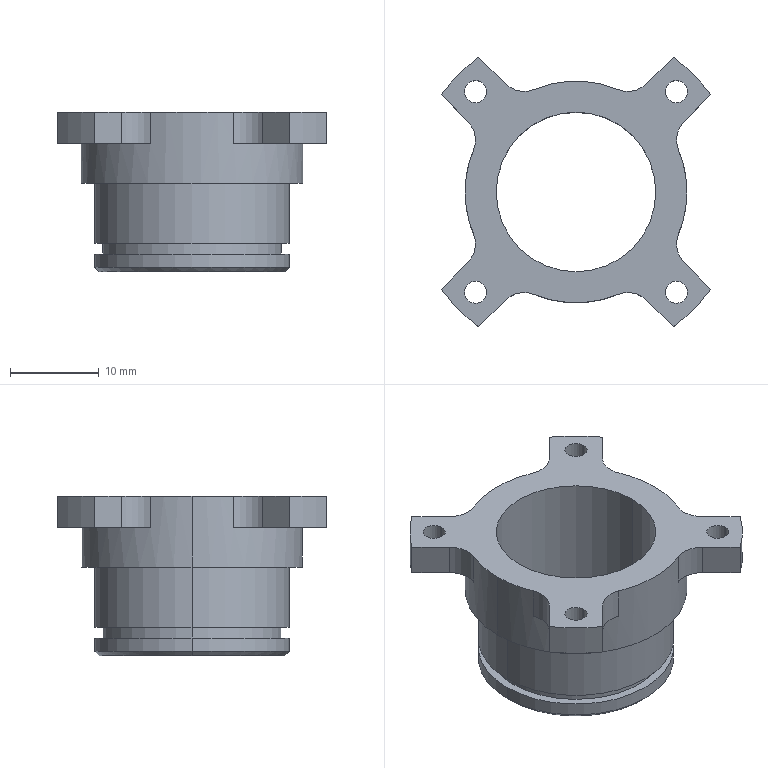Part | SolidWorks | features ICE 6, Chamfer 2, CoordSys 1, Extrusion 1, Fillet 1, HoleWzd 1 | 1 solid | 51 faces | box 30.418 x 30.418 x 18 mm | volume 3548 mm3 | cylinder 32 | plane 17 | cone 2 | commonest cylinder face diameters 6 x10 2.5 x8 22 x4 37.5 x4 18 x2 20.15 x2